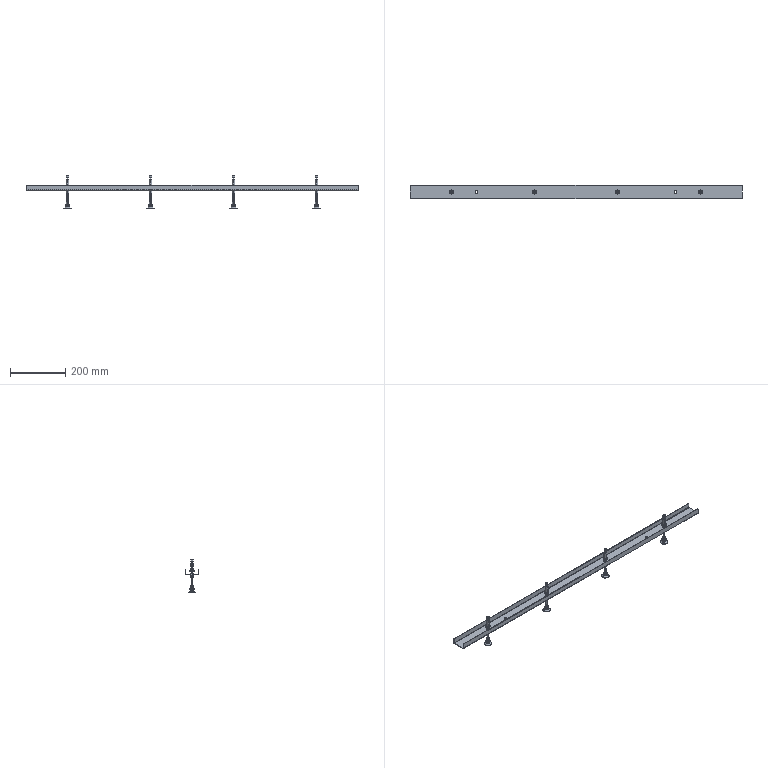Part | SolidWorks | features ReferencePattern 3, LocalLPattern 1 | 13 solids | 678 faces | box 1200 x 50 x 118 mm | volume 235695 mm3 | cone 308 | plane 198 | cylinder 148 | spline 24 | commonest cylinder face diameters 6 x18 5 x16 7 x16 10 x16 4 x12 2 x10